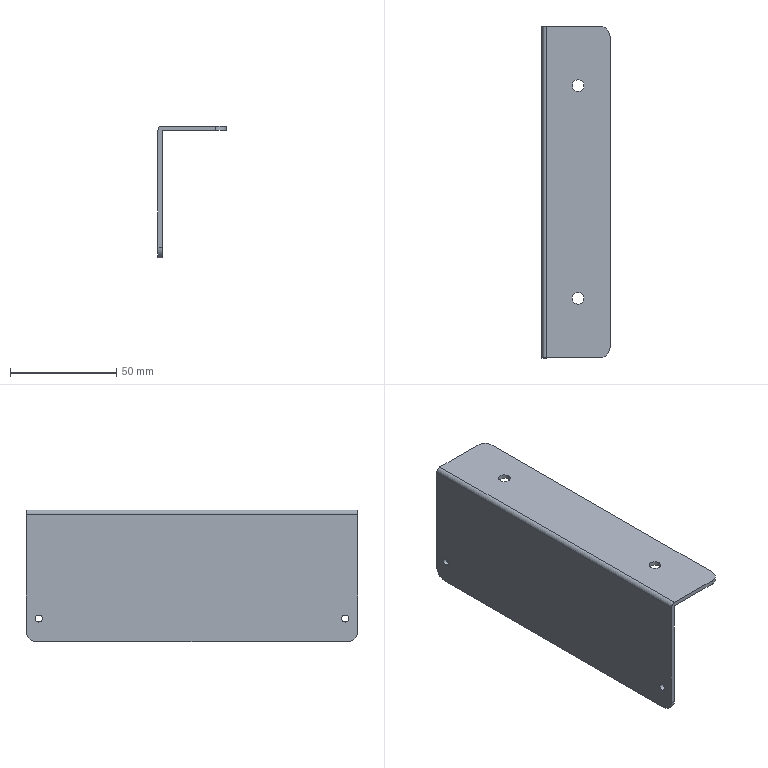Part | STEP file | ND25021-01-JDKM-06-BJ | 1 solid | 21 faces | box 32 x 156 x 62 mm | volume 28398 mm3 | cylinder 13 | plane 8 | commonest cylinder face diameters 3.3 x4 5.5 x4 10 x4 4 x1